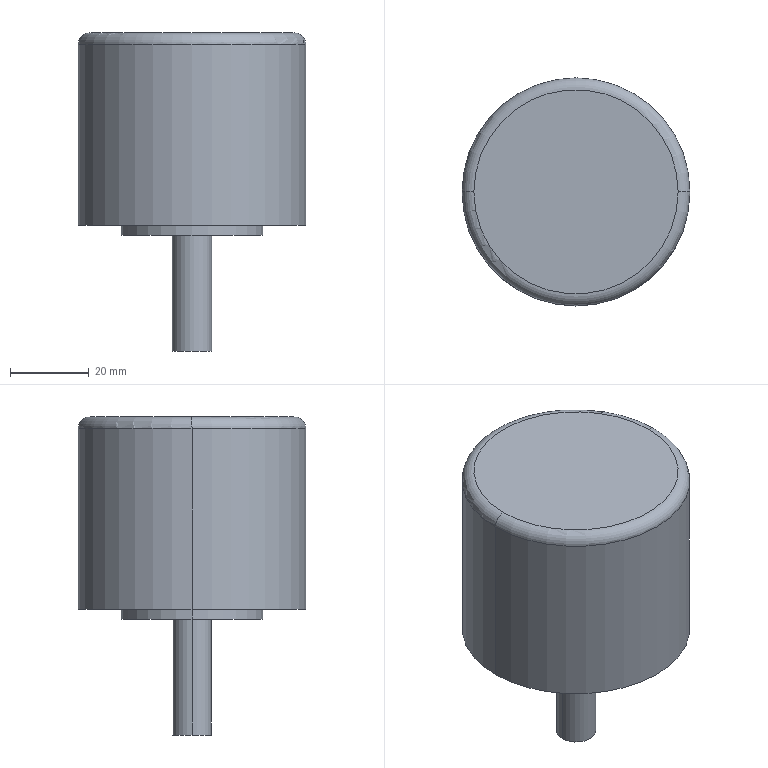Part | SolidWorks | features ICE 2, CirPattern 1, Extrusion 1, Fillet 1, HoleWzd 1 | 1 solid | 24 faces | box 58 x 58 x 81 mm | volume 133866 mm3 | cylinder 12 | cone 6 | plane 4 | torus 2 | commonest cylinder face diameters 2.5 x6 10 x2 36 x2 58 x2
STEP:
#1=CARTESIAN_POINT('',(-5.,0.,-56.5));
#2=VERTEX_POINT('',#1);
#3=CARTESIAN_POINT('',(5.,0.,-56.5));
#4=VERTEX_POINT('',#3);
#5=CARTESIAN_POINT('',(0.,0.,-56.5));
#6=DIRECTION('',(0.,0.,-1.));
#7=DIRECTION('',(-1.,0.,0.));
#8=AXIS2_PLACEMENT_3D('',#5,#6,#7);
#9=CIRCLE('',#8,5.);
#10=EDGE_CURVE('',#2,#4,#9,.T.);
#11=ORIENTED_EDGE('',*,*,#10,.F.);
#12=CARTESIAN_POINT('',(-5.,0.,-27.));
#13=VERTEX_POINT('',#12);
#14=CARTESIAN_POINT('',(-5.,0.,-56.5));
#15=DIRECTION('',(0.,0.,1.));
#16=VECTOR('',#15,1000.);
#17=LINE('',#14,#16);
#18=EDGE_CURVE('',#2,#13,#17,.T.);
#19=ORIENTED_EDGE('',*,*,#18,.T.);
#20=CARTESIAN_POINT('',(5.,0.,-27.));
#21=VERTEX_POINT('',#20);
#22=CARTESIAN_POINT('',(0.,0.,-27.));
#23=DIRECTION('',(0.,0.,-1.));
#24=DIRECTION('',(-1.,0.,0.));
#25=AXIS2_PLACEMENT_3D('',#22,#23,#24);
#26=CIRCLE('',#25,5.);
#27=EDGE_CURVE('',#13,#21,#26,.T.);
#28=ORIENTED_EDGE('',*,*,#27,.T.);
#29=CARTESIAN_POINT('',(5.,0.,-56.5));
#30=DIRECTION('',(0.,0.,1.));
#31=VECTOR('',#30,1000.);
#32=LINE('',#29,#31);
#33=EDGE_CURVE('',#4,#21,#32,.T.);
#34=ORIENTED_EDGE('',*,*,#33,.F.);
#35=EDGE_LOOP('',(#11,#19,#28,#34));
#36=FACE_OUTER_BOUND('',#35,.T.);
#37=CARTESIAN_POINT('',(0.,0.,-56.5));
#38=DIRECTION('',(0.,0.,1.));
#39=DIRECTION('',(1.,0.,0.));
#40=AXIS2_PLACEMENT_3D('',#37,#38,#39);
#41=CYLINDRICAL_SURFACE('',#40,5.);
#42=ADVANCED_FACE('',(#36),#41,.T.);
#43=CARTESIAN_POINT('',(-18.,0.,-27.));
#44=VERTEX_POINT('',#43);
#45=CARTESIAN_POINT('',(18.,0.,-27.));
#46=VERTEX_POINT('',#45);
#47=CARTESIAN_POINT('',(0.,0.,-27.));
#48=DIRECTION('',(0.,0.,-1.));
#49=DIRECTION('',(-1.,0.,0.));
#50=AXIS2_PLACEMENT_3D('',#47,#48,#49);
#51=CIRCLE('',#50,18.);
#52=EDGE_CURVE('',#44,#46,#51,.T.);
#53=ORIENTED_EDGE('',*,*,#52,.F.);
#54=CARTESIAN_POINT('',(-18.,0.,-24.5));
#55=VERTEX_POINT('',#54);
#56=CARTESIAN_POINT('',(-18.,0.,-27.));
#57=DIRECTION('',(0.,0.,1.));
#58=VECTOR('',#57,1000.);
#59=LINE('',#56,#58);
#60=EDGE_CURVE('',#44,#55,#59,.T.);
#61=ORIENTED_EDGE('',*,*,#60,.T.);
#62=CARTESIAN_POINT('',(18.,0.,-24.5));
#63=VERTEX_POINT('',#62);
#64=CARTESIAN_POINT('',(0.,0.,-24.5));
#65=DIRECTION('',(0.,0.,-1.));
#66=DIRECTION('',(1.,0.,0.));
#67=AXIS2_PLACEMENT_3D('',#64,#65,#66);
#68=CIRCLE('',#67,18.);
#69=EDGE_CURVE('',#55,#63,#68,.T.);
#70=ORIENTED_EDGE('',*,*,#69,.T.);
#71=CARTESIAN_POINT('',(18.,0.,-27.));
#72=DIRECTION('',(0.,0.,1.));
#73=VECTOR('',#72,1000.);
#74=LINE('',#71,#73);
#75=EDGE_CURVE('',#46,#63,#74,.T.);
#76=ORIENTED_EDGE('',*,*,#75,.F.);
#77=EDGE_LOOP('',(#53,#61,#70,#76));
#78=FACE_OUTER_BOUND('',#77,.T.);
#79=CARTESIAN_POINT('',(0.,0.,-27.));
#80=DIRECTION('',(0.,0.,1.));
#81=DIRECTION('',(1.,0.,0.));
#82=AXIS2_PLACEMENT_3D('',#79,#80,#81);
#83=CYLINDRICAL_SURFACE('',#82,18.);
#84=ADVANCED_FACE('',(#78),#83,.T.);
#85=CARTESIAN_POINT('',(13.25,-20.785,-17.));
#86=VERTEX_POINT('',#85);
#87=CARTESIAN_POINT('',(10.75,-20.785,-17.));
#88=VERTEX_POINT('',#87);
#89=CARTESIAN_POINT('',(12.,-20.785,-17.));
#90=DIRECTION('',(0.,0.,-1.));
#91=DIRECTION('',(-1.,0.,0.));
#92=AXIS2_PLACEMENT_3D('',#89,#90,#91);
#93=CIRCLE('',#92,1.25);
#94=EDGE_CURVE('',#86,#88,#93,.T.);
#95=ORIENTED_EDGE('',*,*,#94,.F.);
#96=CARTESIAN_POINT('',(13.25,-20.785,-24.5));
#97=VERTEX_POINT('',#96);
#98=CARTESIAN_POINT('',(13.25,-20.785,-24.5));
#99=DIRECTION('',(0.,0.,-1.));
#100=VECTOR('',#99,1000.);
#101=LINE('',#98,#100);
#102=EDGE_CURVE('',#86,#97,#101,.T.);
#103=ORIENTED_EDGE('',*,*,#102,.T.);
#104=CARTESIAN_POINT('',(10.75,-20.785,-24.5));
#105=VERTEX_POINT('',#104);
#106=CARTESIAN_POINT('',(12.,-20.785,-24.5));
#107=DIRECTION('',(0.,0.,-1.));
#108=DIRECTION('',(-1.,0.,0.));
#109=AXIS2_PLACEMENT_3D('',#106,#107,#108);
#110=CIRCLE('',#109,1.25);
#111=EDGE_CURVE('',#97,#105,#110,.T.);
#112=ORIENTED_EDGE('',*,*,#111,.T.);
#113=CARTESIAN_POINT('',(10.75,-20.785,-24.5));
#114=DIRECTION('',(0.,0.,-1.));
#115=VECTOR('',#114,1000.);
#116=LINE('',#113,#115);
#117=EDGE_CURVE('',#88,#105,#116,.T.);
#118=ORIENTED_EDGE('',*,*,#117,.F.);
#119=EDGE_LOOP('',(#95,#103,#112,#118));
#120=FACE_OUTER_BOUND('',#119,.T.);
#121=CARTESIAN_POINT('',(12.,-20.785,-24.5));
#122=DIRECTION('',(0.,0.,-1.));
#123=DIRECTION('',(-1.,0.,0.));
#124=AXIS2_PLACEMENT_3D('',#121,#122,#123);
#125=CYLINDRICAL_SURFACE('',#124,1.25);
#126=ADVANCED_FACE('',(#120),#125,.F.);
#127=CARTESIAN_POINT('',(12.,-20.785,-16.249));
#128=VERTEX_POINT('',#127);
#129=CARTESIAN_POINT('',(10.75,-20.785,-17.));
#130=DIRECTION('',(-0.8572,0.,-0.515));
#131=VECTOR('',#130,1000.);
#132=LINE('',#129,#131);
#133=EDGE_CURVE('',#128,#88,#132,.T.);
#134=ORIENTED_EDGE('',*,*,#133,.F.);
#135=CARTESIAN_POINT('',(13.25,-20.785,-17.));
#136=DIRECTION('',(0.8572,0.,-0.515));
#137=VECTOR('',#136,1000.);
#138=LINE('',#135,#137);
#139=EDGE_CURVE('',#128,#86,#138,.T.);
#140=ORIENTED_EDGE('',*,*,#139,.T.);
#141=ORIENTED_EDGE('',*,*,#94,.T.);
#142=EDGE_LOOP('',(#134,#140,#141));
#143=FACE_OUTER_BOUND('',#142,.T.);
#144=CARTESIAN_POINT('',(12.,-20.785,-17.));
#145=DIRECTION('',(0.,0.,-1.));
#146=DIRECTION('',(-1.,0.,0.));
#147=AXIS2_PLACEMENT_3D('',#144,#145,#146);
#148=CONICAL_SURFACE('',#147,1.25,1.03);
#149=ADVANCED_FACE('',(#143),#148,.F.);
#150=CARTESIAN_POINT('',(13.25,20.785,-17.));
#151=VERTEX_POINT('',#150);
#152=CARTESIAN_POINT('',(10.75,20.785,-17.));
#153=VERTEX_POINT('',#152);
#154=CARTESIAN_POINT('',(12.,20.785,-17.));
#155=DIRECTION('',(0.,0.,-1.));
#156=DIRECTION('',(-1.,0.,0.));
#157=AXIS2_PLACEMENT_3D('',#154,#155,#156);
#158=CIRCLE('',#157,1.25);
#159=EDGE_CURVE('',#151,#153,#158,.T.);
#160=ORIENTED_EDGE('',*,*,#159,.F.);
#161=CARTESIAN_POINT('',(13.25,20.785,-24.5));
#162=VERTEX_POINT('',#161);
#163=CARTESIAN_POINT('',(13.25,20.785,-24.5));
#164=DIRECTION('',(0.,0.,-1.));
#165=VECTOR('',#164,1000.);
#166=LINE('',#163,#165);
#167=EDGE_CURVE('',#151,#162,#166,.T.);
#168=ORIENTED_EDGE('',*,*,#167,.T.);
#169=CARTESIAN_POINT('',(10.75,20.785,-24.5));
#170=VERTEX_POINT('',#169);
#171=CARTESIAN_POINT('',(12.,20.785,-24.5));
#172=DIRECTION('',(0.,0.,-1.));
#173=DIRECTION('',(-1.,0.,0.));
#174=AXIS2_PLACEMENT_3D('',#171,#172,#173);
#175=CIRCLE('',#174,1.25);
#176=EDGE_CURVE('',#162,#170,#175,.T.);
#177=ORIENTED_EDGE('',*,*,#176,.T.);
#178=CARTESIAN_POINT('',(10.75,20.785,-24.5));
#179=DIRECTION('',(0.,0.,-1.));
#180=VECTOR('',#179,1000.);
#181=LINE('',#178,#180);
#182=EDGE_CURVE('',#153,#170,#181,.T.);
#183=ORIENTED_EDGE('',*,*,#182,.F.);
#184=EDGE_LOOP('',(#160,#168,#177,#183));
#185=FACE_OUTER_BOUND('',#184,.T.);
#186=CARTESIAN_POINT('',(12.,20.785,-24.5));
#187=DIRECTION('',(0.,0.,-1.));
#188=DIRECTION('',(-1.,0.,0.));
#189=AXIS2_PLACEMENT_3D('',#186,#187,#188);
#190=CYLINDRICAL_SURFACE('',#189,1.25);
#191=ADVANCED_FACE('',(#185),#190,.F.);
#192=CARTESIAN_POINT('',(12.,20.785,-16.249));
#193=VERTEX_POINT('',#192);
#194=CARTESIAN_POINT('',(10.75,20.785,-17.));
#195=DIRECTION('',(-0.8572,0.,-0.515));
#196=VECTOR('',#195,1000.);
#197=LINE('',#194,#196);
#198=EDGE_CURVE('',#193,#153,#197,.T.);
#199=ORIENTED_EDGE('',*,*,#198,.F.);
#200=CARTESIAN_POINT('',(13.25,20.785,-17.));
#201=DIRECTION('',(0.8572,0.,-0.515));
#202=VECTOR('',#201,1000.);
#203=LINE('',#200,#202);
#204=EDGE_CURVE('',#193,#151,#203,.T.);
#205=ORIENTED_EDGE('',*,*,#204,.T.);
#206=ORIENTED_EDGE('',*,*,#159,.T.);
#207=EDGE_LOOP('',(#199,#205,#206));
#208=FACE_OUTER_BOUND('',#207,.T.);
#209=CARTESIAN_POINT('',(12.,20.785,-17.));
#210=DIRECTION('',(0.,0.,-1.));
#211=DIRECTION('',(-1.,0.,0.));
#212=AXIS2_PLACEMENT_3D('',#209,#210,#211);
#213=CONICAL_SURFACE('',#212,1.25,1.03);
#214=ADVANCED_FACE('',(#208),#213,.F.);
#215=CARTESIAN_POINT('',(-22.75,0.,-17.));
#216=VERTEX_POINT('',#215);
#217=CARTESIAN_POINT('',(-25.25,0.,-17.));
#218=VERTEX_POINT('',#217);
#219=CARTESIAN_POINT('',(-24.,0.,-17.));
#220=DIRECTION('',(0.,0.,-1.));
#221=DIRECTION('',(-1.,0.,0.));
#222=AXIS2_PLACEMENT_3D('',#219,#220,#221);
#223=CIRCLE('',#222,1.25);
#224=EDGE_CURVE('',#216,#218,#223,.T.);
#225=ORIENTED_EDGE('',*,*,#224,.F.);
#226=CARTESIAN_POINT('',(-22.75,0.,-24.5));
#227=VERTEX_POINT('',#226);
#228=CARTESIAN_POINT('',(-22.75,0.,-24.5));
#229=DIRECTION('',(0.,0.,-1.));
#230=VECTOR('',#229,1000.);
#231=LINE('',#228,#230);
#232=EDGE_CURVE('',#216,#227,#231,.T.);
#233=ORIENTED_EDGE('',*,*,#232,.T.);
#234=CARTESIAN_POINT('',(-25.25,0.,-24.5));
#235=VERTEX_POINT('',#234);
#236=CARTESIAN_POINT('',(-24.,0.,-24.5));
#237=DIRECTION('',(0.,0.,-1.));
#238=DIRECTION('',(-1.,0.,0.));
#239=AXIS2_PLACEMENT_3D('',#236,#237,#238);
#240=CIRCLE('',#239,1.25);
#241=EDGE_CURVE('',#227,#235,#240,.T.);
#242=ORIENTED_EDGE('',*,*,#241,.T.);
#243=CARTESIAN_POINT('',(-25.25,0.,-24.5));
#244=DIRECTION('',(0.,0.,-1.));
#245=VECTOR('',#244,1000.);
#246=LINE('',#243,#245);
#247=EDGE_CURVE('',#218,#235,#246,.T.);
#248=ORIENTED_EDGE('',*,*,#247,.F.);
#249=EDGE_LOOP('',(#225,#233,#242,#248));
#250=FACE_OUTER_BOUND('',#249,.T.);
#251=CARTESIAN_POINT('',(-24.,0.,-24.5));
#252=DIRECTION('',(0.,0.,-1.));
#253=DIRECTION('',(-1.,0.,0.));
#254=AXIS2_PLACEMENT_3D('',#251,#252,#253);
#255=CYLINDRICAL_SURFACE('',#254,1.25);
#256=ADVANCED_FACE('',(#250),#255,.F.);
#257=CARTESIAN_POINT('',(-24.,0.,-16.249));
#258=VERTEX_POINT('',#257);
#259=CARTESIAN_POINT('',(-25.25,0.,-17.));
#260=DIRECTION('',(-0.8572,0.,-0.515));
#261=VECTOR('',#260,1000.);
#262=LINE('',#259,#261);
#263=EDGE_CURVE('',#258,#218,#262,.T.);
#264=ORIENTED_EDGE('',*,*,#263,.F.);
#265=CARTESIAN_POINT('',(-22.75,0.,-17.));
#266=DIRECTION('',(0.8572,0.,-0.515));
#267=VECTOR('',#266,1000.);
#268=LINE('',#265,#267);
#269=EDGE_CURVE('',#258,#216,#268,.T.);
#270=ORIENTED_EDGE('',*,*,#269,.T.);
#271=ORIENTED_EDGE('',*,*,#224,.T.);
#272=EDGE_LOOP('',(#264,#270,#271));
#273=FACE_OUTER_BOUND('',#272,.T.);
#274=CARTESIAN_POINT('',(-24.,0.,-17.));
#275=DIRECTION('',(0.,0.,-1.));
#276=DIRECTION('',(-1.,0.,0.));
#277=AXIS2_PLACEMENT_3D('',#274,#275,#276);
#278=CONICAL_SURFACE('',#277,1.25,1.03);
#279=ADVANCED_FACE('',(#273),#278,.F.);
#280=CARTESIAN_POINT('',(-29.,0.,21.5));
#281=VERTEX_POINT('',#280);
#282=CARTESIAN_POINT('',(29.,0.,21.5));
#283=VERTEX_POINT('',#282);
#284=CARTESIAN_POINT('',(0.,0.,21.5));
#285=DIRECTION('',(0.,0.,-1.));
#286=DIRECTION('',(1.,0.,0.));
#287=AXIS2_PLACEMENT_3D('',#284,#285,#286);
#288=CIRCLE('',#287,29.);
#289=EDGE_CURVE('',#281,#283,#288,.T.);
#290=ORIENTED_EDGE('',*,*,#289,.F.);
#291=CARTESIAN_POINT('',(-26.,0.,24.5));
#292=VERTEX_POINT('',#291);
#293=CARTESIAN_POINT('',(-26.,0.,21.5));
#294=DIRECTION('',(0.,1.,0.));
#295=DIRECTION('',(-1.,0.,0.));
#296=AXIS2_PLACEMENT_3D('',#293,#294,#295);
#297=CIRCLE('',#296,3.);
#298=EDGE_CURVE('',#281,#292,#297,.T.);
#299=ORIENTED_EDGE('',*,*,#298,.T.);
#300=CARTESIAN_POINT('',(26.,0.,24.5));
#301=VERTEX_POINT('',#300);
#302=CARTESIAN_POINT('',(0.,0.,24.5));
#303=DIRECTION('',(0.,0.,1.));
#304=DIRECTION('',(1.,0.,0.));
#305=AXIS2_PLACEMENT_3D('',#302,#303,#304);
#306=CIRCLE('',#305,26.);
#307=EDGE_CURVE('',#301,#292,#306,.T.);
#308=ORIENTED_EDGE('',*,*,#307,.F.);
#309=CARTESIAN_POINT('',(26.,0.,21.5));
#310=DIRECTION('',(0.,-1.,0.));
#311=DIRECTION('',(0.,0.,-1.));
#312=AXIS2_PLACEMENT_3D('',#309,#310,#311);
#313=CIRCLE('',#312,3.);
#314=EDGE_CURVE('',#283,#301,#313,.T.);
#315=ORIENTED_EDGE('',*,*,#314,.F.);
#316=EDGE_LOOP('',(#290,#299,#308,#315));
#317=FACE_OUTER_BOUND('',#316,.T.);
#318=CARTESIAN_POINT('',(0.,0.,21.5));
#319=DIRECTION('',(0.,0.,1.));
#320=DIRECTION('',(1.,0.,0.));
#321=AXIS2_PLACEMENT_3D('',#318,#319,#320);
#322=TOROIDAL_SURFACE('',#321,26.,3.);
#323=ADVANCED_FACE('',(#317),#322,.T.);
#324=ORIENTED_EDGE('',*,*,#289,.T.);
#325=CARTESIAN_POINT('',(29.,0.,-24.5));
#326=VERTEX_POINT('',#325);
#327=CARTESIAN_POINT('',(29.,0.,24.5));
#328=DIRECTION('',(0.,0.,-1.));
#329=VECTOR('',#328,1000.);
#330=LINE('',#327,#329);
#331=EDGE_CURVE('',#283,#326,#330,.T.);
#332=ORIENTED_EDGE('',*,*,#331,.T.);
#333=CARTESIAN_POINT('',(-29.,0.,-24.5));
#334=VERTEX_POINT('',#333);
#335=CARTESIAN_POINT('',(0.,0.,-24.5));
#336=DIRECTION('',(0.,0.,1.));
#337=DIRECTION('',(1.,0.,0.));
#338=AXIS2_PLACEMENT_3D('',#335,#336,#337);
#339=CIRCLE('',#338,29.);
#340=EDGE_CURVE('',#326,#334,#339,.T.);
#341=ORIENTED_EDGE('',*,*,#340,.T.);
#342=CARTESIAN_POINT('',(-29.,0.,24.5));
#343=DIRECTION('',(0.,0.,-1.));
#344=VECTOR('',#343,1000.);
#345=LINE('',#342,#344);
#346=EDGE_CURVE('',#281,#334,#345,.T.);
#347=ORIENTED_EDGE('',*,*,#346,.F.);
#348=EDGE_LOOP('',(#324,#332,#341,#347));
#349=FACE_OUTER_BOUND('',#348,.T.);
#350=CARTESIAN_POINT('',(0.,0.,24.5));
#351=DIRECTION('',(0.,0.,-1.));
#352=DIRECTION('',(-1.,0.,0.));
#353=AXIS2_PLACEMENT_3D('',#350,#351,#352);
#354=CYLINDRICAL_SURFACE('',#353,29.);
#355=ADVANCED_FACE('',(#349),#354,.T.);
#356=CARTESIAN_POINT('',(0.,0.,-24.5));
#357=DIRECTION('',(0.,0.,1.));
#358=DIRECTION('',(1.,0.,0.));
#359=AXIS2_PLACEMENT_3D('',#356,#357,#358);
#360=CIRCLE('',#359,29.);
#361=EDGE_CURVE('',#334,#326,#360,.T.);
#362=ORIENTED_EDGE('',*,*,#361,.F.);
#363=ORIENTED_EDGE('',*,*,#340,.F.);
#364=EDGE_LOOP('',(#362,#363));
#365=FACE_OUTER_BOUND('',#364,.T.);
#366=CARTESIAN_POINT('',(-24.,0.,-24.5));
#367=DIRECTION('',(0.,0.,-1.));
#368=DIRECTION('',(-1.,0.,0.));
#369=AXIS2_PLACEMENT_3D('',#366,#367,#368);
#370=CIRCLE('',#369,1.25);
#371=EDGE_CURVE('',#235,#227,#370,.T.);
#372=ORIENTED_EDGE('',*,*,#371,.F.);
#373=ORIENTED_EDGE('',*,*,#241,.F.);
#374=EDGE_LOOP('',(#372,#373));
#375=FACE_BOUND('',#374,.T.);
#376=CARTESIAN_POINT('',(12.,20.785,-24.5));
#377=DIRECTION('',(0.,0.,-1.));
#378=DIRECTION('',(-1.,0.,0.));
#379=AXIS2_PLACEMENT_3D('',#376,#377,#378);
#380=CIRCLE('',#379,1.25);
#381=EDGE_CURVE('',#170,#162,#380,.T.);
#382=ORIENTED_EDGE('',*,*,#381,.F.);
#383=ORIENTED_EDGE('',*,*,#176,.F.);
#384=EDGE_LOOP('',(#382,#383));
#385=FACE_BOUND('',#384,.T.);
#386=CARTESIAN_POINT('',(12.,-20.785,-24.5));
#387=DIRECTION('',(0.,0.,-1.));
#388=DIRECTION('',(-1.,0.,0.));
#389=AXIS2_PLACEMENT_3D('',#386,#387,#388);
#390=CIRCLE('',#389,1.25);
#391=EDGE_CURVE('',#105,#97,#390,.T.);
#392=ORIENTED_EDGE('',*,*,#391,.F.);
#393=ORIENTED_EDGE('',*,*,#111,.F.);
#394=EDGE_LOOP('',(#392,#393));
#395=FACE_BOUND('',#394,.T.);
#396=CARTESIAN_POINT('',(0.,0.,-24.5));
#397=DIRECTION('',(0.,0.,-1.));
#398=DIRECTION('',(1.,0.,0.));
#399=AXIS2_PLACEMENT_3D('',#396,#397,#398);
#400=CIRCLE('',#399,18.);
#401=EDGE_CURVE('',#63,#55,#400,.T.);
#402=ORIENTED_EDGE('',*,*,#401,.F.);
#403=ORIENTED_EDGE('',*,*,#69,.F.);
#404=EDGE_LOOP('',(#402,#403));
#405=FACE_BOUND('',#404,.T.);
#406=CARTESIAN_POINT('',(0.,0.,-24.5));
#407=DIRECTION('',(0.,0.,1.));
#408=DIRECTION('',(1.,0.,0.));
#409=AXIS2_PLACEMENT_3D('',#406,#407,#408);
#410=PLANE('',#409);
#411=ADVANCED_FACE('',(#365,#375,#385,#395,#405),#410,.F.);
#412=ORIENTED_EDGE('',*,*,#331,.F.);
#413=CARTESIAN_POINT('',(0.,0.,21.5));
#414=DIRECTION('',(0.,0.,-1.));
#415=DIRECTION('',(1.,0.,0.));
#416=AXIS2_PLACEMENT_3D('',#413,#414,#415);
#417=CIRCLE('',#416,29.);
#418=EDGE_CURVE('',#283,#281,#417,.T.);
#419=ORIENTED_EDGE('',*,*,#418,.T.);
#420=ORIENTED_EDGE('',*,*,#346,.T.);
#421=ORIENTED_EDGE('',*,*,#361,.T.);
#422=EDGE_LOOP('',(#412,#419,#420,#421));
#423=FACE_OUTER_BOUND('',#422,.T.);
#424=CARTESIAN_POINT('',(0.,0.,24.5));
#425=DIRECTION('',(0.,0.,-1.));
#426=DIRECTION('',(-1.,0.,0.));
#427=AXIS2_PLACEMENT_3D('',#424,#425,#426);
#428=CYLINDRICAL_SURFACE('',#427,29.);
#429=ADVANCED_FACE('',(#423),#428,.T.);
#430=ORIENTED_EDGE('',*,*,#307,.T.);
#431=CARTESIAN_POINT('',(0.,0.,24.5));
#432=DIRECTION('',(0.,0.,1.));
#433=DIRECTION('',(1.,0.,0.));
#434=AXIS2_PLACEMENT_3D('',#431,#432,#433);
#435=CIRCLE('',#434,26.);
#436=EDGE_CURVE('',#292,#301,#435,.T.);
#437=ORIENTED_EDGE('',*,*,#436,.T.);
#438=EDGE_LOOP('',(#430,#437));
#439=FACE_OUTER_BOUND('',#438,.T.);
#440=CARTESIAN_POINT('',(0.,0.,24.5));
#441=DIRECTION('',(0.,0.,1.));
#442=DIRECTION('',(1.,0.,0.));
#443=AXIS2_PLACEMENT_3D('',#440,#441,#442);
#444=PLANE('',#443);
#445=ADVANCED_FACE('',(#439),#444,.T.);
#446=ORIENTED_EDGE('',*,*,#298,.F.);
#447=ORIENTED_EDGE('',*,*,#418,.F.);
#448=ORIENTED_EDGE('',*,*,#314,.T.);
#449=ORIENTED_EDGE('',*,*,#436,.F.);
#450=EDGE_LOOP('',(#446,#447,#448,#449));
#451=FACE_OUTER_BOUND('',#450,.T.);
#452=CARTESIAN_POINT('',(0.,0.,21.5));
#453=DIRECTION('',(0.,0.,1.));
#454=DIRECTION('',(1.,0.,0.));
#455=AXIS2_PLACEMENT_3D('',#452,#453,#454);
#456=TOROIDAL_SURFACE('',#455,26.,3.);
#457=ADVANCED_FACE('',(#451),#456,.T.);
#458=ORIENTED_EDGE('',*,*,#269,.F.);
#459=ORIENTED_EDGE('',*,*,#263,.T.);
#460=CARTESIAN_POINT('',(-24.,0.,-17.));
#461=DIRECTION('',(0.,0.,-1.));
#462=DIRECTION('',(-1.,0.,0.));
#463=AXIS2_PLACEMENT_3D('',#460,#461,#462);
#464=CIRCLE('',#463,1.25);
#465=EDGE_CURVE('',#218,#216,#464,.T.);
#466=ORIENTED_EDGE('',*,*,#465,.T.);
#467=EDGE_LOOP('',(#458,#459,#466));
#468=FACE_OUTER_BOUND('',#467,.T.);
#469=CARTESIAN_POINT('',(-24.,0.,-17.));
#470=DIRECTION('',(0.,0.,-1.));
#471=DIRECTION('',(-1.,0.,0.));
#472=AXIS2_PLACEMENT_3D('',#469,#470,#471);
#473=CONICAL_SURFACE('',#472,1.25,1.03);
#474=ADVANCED_FACE('',(#468),#473,.F.);
#475=ORIENTED_EDGE('',*,*,#232,.F.);
#476=ORIENTED_EDGE('',*,*,#465,.F.);
#477=ORIENTED_EDGE('',*,*,#247,.T.);
#478=ORIENTED_EDGE('',*,*,#371,.T.);
#479=EDGE_LOOP('',(#475,#476,#477,#478));
#480=FACE_OUTER_BOUND('',#479,.T.);
#481=CARTESIAN_POINT('',(-24.,0.,-24.5));
#482=DIRECTION('',(0.,0.,-1.));
#483=DIRECTION('',(-1.,0.,0.));
#484=AXIS2_PLACEMENT_3D('',#481,#482,#483);
#485=CYLINDRICAL_SURFACE('',#484,1.25);
#486=ADVANCED_FACE('',(#480),#485,.F.);
#487=ORIENTED_EDGE('',*,*,#204,.F.);
#488=ORIENTED_EDGE('',*,*,#198,.T.);
#489=CARTESIAN_POINT('',(12.,20.785,-17.));
#490=DIRECTION('',(0.,0.,-1.));
#491=DIRECTION('',(-1.,0.,0.));
#492=AXIS2_PLACEMENT_3D('',#489,#490,#491);
#493=CIRCLE('',#492,1.25);
#494=EDGE_CURVE('',#153,#151,#493,.T.);
#495=ORIENTED_EDGE('',*,*,#494,.T.);
#496=EDGE_LOOP('',(#487,#488,#495));
#497=FACE_OUTER_BOUND('',#496,.T.);
#498=CARTESIAN_POINT('',(12.,20.785,-17.));
#499=DIRECTION('',(0.,0.,-1.));
#500=DIRECTION('',(-1.,0.,0.));
#501=AXIS2_PLACEMENT_3D('',#498,#499,#500);
#502=CONICAL_SURFACE('',#501,1.25,1.03);
#503=ADVANCED_FACE('',(#497),#502,.F.);
#504=ORIENTED_EDGE('',*,*,#167,.F.);
#505=ORIENTED_EDGE('',*,*,#494,.F.);
#506=ORIENTED_EDGE('',*,*,#182,.T.);
#507=ORIENTED_EDGE('',*,*,#381,.T.);
#508=EDGE_LOOP('',(#504,#505,#506,#507));
#509=FACE_OUTER_BOUND('',#508,.T.);
#510=CARTESIAN_POINT('',(12.,20.785,-24.5));
#511=DIRECTION('',(0.,0.,-1.));
#512=DIRECTION('',(-1.,0.,0.));
#513=AXIS2_PLACEMENT_3D('',#510,#511,#512);
#514=CYLINDRICAL_SURFACE('',#513,1.25);
#515=ADVANCED_FACE('',(#509),#514,.F.);
#516=ORIENTED_EDGE('',*,*,#139,.F.);
#517=ORIENTED_EDGE('',*,*,#133,.T.);
#518=CARTESIAN_POINT('',(12.,-20.785,-17.));
#519=DIRECTION('',(0.,0.,-1.));
#520=DIRECTION('',(-1.,0.,0.));
#521=AXIS2_PLACEMENT_3D('',#518,#519,#520);
#522=CIRCLE('',#521,1.25);
#523=EDGE_CURVE('',#88,#86,#522,.T.);
#524=ORIENTED_EDGE('',*,*,#523,.T.);
#525=EDGE_LOOP('',(#516,#517,#524));
#526=FACE_OUTER_BOUND('',#525,.T.);
#527=CARTESIAN_POINT('',(12.,-20.785,-17.));
#528=DIRECTION('',(0.,0.,-1.));
#529=DIRECTION('',(-1.,0.,0.));
#530=AXIS2_PLACEMENT_3D('',#527,#528,#529);
#531=CONICAL_SURFACE('',#530,1.25,1.03);
#532=ADVANCED_FACE('',(#526),#531,.F.);
#533=ORIENTED_EDGE('',*,*,#102,.F.);
#534=ORIENTED_EDGE('',*,*,#523,.F.);
#535=ORIENTED_EDGE('',*,*,#117,.T.);
#536=ORIENTED_EDGE('',*,*,#391,.T.);
#537=EDGE_LOOP('',(#533,#534,#535,#536));
#538=FACE_OUTER_BOUND('',#537,.T.);
#539=CARTESIAN_POINT('',(12.,-20.785,-24.5));
#540=DIRECTION('',(0.,0.,-1.));
#541=DIRECTION('',(-1.,0.,0.));
#542=AXIS2_PLACEMENT_3D('',#539,#540,#541);
#543=CYLINDRICAL_SURFACE('',#542,1.25);
#544=ADVANCED_FACE('',(#538),#543,.F.);
#545=CARTESIAN_POINT('',(0.,0.,-27.));
#546=DIRECTION('',(0.,0.,-1.));
#547=DIRECTION('',(-1.,0.,0.));
#548=AXIS2_PLACEMENT_3D('',#545,#546,#547);
#549=CIRCLE('',#548,18.);
#550=EDGE_CURVE('',#46,#44,#549,.T.);
#551=ORIENTED_EDGE('',*,*,#550,.T.);
#552=ORIENTED_EDGE('',*,*,#52,.T.);
#553=EDGE_LOOP('',(#551,#552));
#554=FACE_OUTER_BOUND('',#553,.T.);
#555=CARTESIAN_POINT('',(0.,0.,-27.));
#556=DIRECTION('',(0.,0.,-1.));
#557=DIRECTION('',(-1.,0.,0.));
#558=AXIS2_PLACEMENT_3D('',#555,#556,#557);
#559=CIRCLE('',#558,5.);
#560=EDGE_CURVE('',#21,#13,#559,.T.);
#561=ORIENTED_EDGE('',*,*,#560,.F.);
#562=ORIENTED_EDGE('',*,*,#27,.F.);
#563=EDGE_LOOP('',(#561,#562));
#564=FACE_BOUND('',#563,.T.);
#565=CARTESIAN_POINT('',(0.,0.,-27.));
#566=DIRECTION('',(0.,0.,-1.));
#567=DIRECTION('',(-1.,0.,0.));
#568=AXIS2_PLACEMENT_3D('',#565,#566,#567);
#569=PLANE('',#568);
#570=ADVANCED_FACE('',(#554,#564),#569,.T.);
#571=ORIENTED_EDGE('',*,*,#60,.F.);
#572=ORIENTED_EDGE('',*,*,#550,.F.);
#573=ORIENTED_EDGE('',*,*,#75,.T.);
#574=ORIENTED_EDGE('',*,*,#401,.T.);
#575=EDGE_LOOP('',(#571,#572,#573,#574));
#576=FACE_OUTER_BOUND('',#575,.T.);
#577=CARTESIAN_POINT('',(0.,0.,-27.));
#578=DIRECTION('',(0.,0.,1.));
#579=DIRECTION('',(1.,0.,0.));
#580=AXIS2_PLACEMENT_3D('',#577,#578,#579);
#581=CYLINDRICAL_SURFACE('',#580,18.);
#582=ADVANCED_FACE('',(#576),#581,.T.);
#583=CARTESIAN_POINT('',(0.,0.,-56.5));
#584=DIRECTION('',(0.,0.,-1.));
#585=DIRECTION('',(-1.,0.,0.));
#586=AXIS2_PLACEMENT_3D('',#583,#584,#585);
#587=CIRCLE('',#586,5.);
#588=EDGE_CURVE('',#4,#2,#587,.T.);
#589=ORIENTED_EDGE('',*,*,#588,.T.);
#590=ORIENTED_EDGE('',*,*,#10,.T.);
#591=EDGE_LOOP('',(#589,#590));
#592=FACE_OUTER_BOUND('',#591,.T.);
#593=CARTESIAN_POINT('',(0.,0.,-56.5));
#594=DIRECTION('',(0.,0.,-1.));
#595=DIRECTION('',(-1.,0.,0.));
#596=AXIS2_PLACEMENT_3D('',#593,#594,#595);
#597=PLANE('',#596);
#598=ADVANCED_FACE('',(#592),#597,.T.);
#599=ORIENTED_EDGE('',*,*,#18,.F.);
#600=ORIENTED_EDGE('',*,*,#588,.F.);
#601=ORIENTED_EDGE('',*,*,#33,.T.);
#602=ORIENTED_EDGE('',*,*,#560,.T.);
#603=EDGE_LOOP('',(#599,#600,#601,#602));
#604=FACE_OUTER_BOUND('',#603,.T.);
#605=CARTESIAN_POINT('',(0.,0.,-56.5));
#606=DIRECTION('',(0.,0.,1.));
#607=DIRECTION('',(1.,0.,0.));
#608=AXIS2_PLACEMENT_3D('',#605,#606,#607);
#609=CYLINDRICAL_SURFACE('',#608,5.);
#610=ADVANCED_FACE('',(#604),#609,.T.);
#611=CLOSED_SHELL('',(#42,#84,#126,#149,#191,#214,#256,#279,#323,#355,#411,#429,#445,#457,#474,#486,#503,#515,#532,#544,#570,#582,#598,#610));
#612=MANIFOLD_SOLID_BREP('',#611);
#613=CARTESIAN_POINT('',(0.,0.,0.));
#614=DIRECTION('',(0.,0.,1.));
#615=DIRECTION('',(1.,0.,0.));
#616=AXIS2_PLACEMENT_3D('',#613,#614,#615);
#617=(LENGTH_UNIT()NAMED_UNIT(*)SI_UNIT(.MILLI.,.METRE.));
#618=UNCERTAINTY_MEASURE_WITH_UNIT(LENGTH_MEASURE(0.00001),#617,'','');
#619=(NAMED_UNIT(*)PLANE_ANGLE_UNIT()SI_UNIT($,.RADIAN.));
#620=(NAMED_UNIT(*)SI_UNIT($,.STERADIAN.)SOLID_ANGLE_UNIT());
#621=(GEOMETRIC_REPRESENTATION_CONTEXT(3)GLOBAL_UNCERTAINTY_ASSIGNED_CONTEXT((#618))GLOBAL_UNIT_ASSIGNED_CONTEXT((#617,#619,#620))REPRESENTATION_CONTEXT('',''));
#622=ADVANCED_BREP_SHAPE_REPRESENTATION('',(#612,#616),#621);